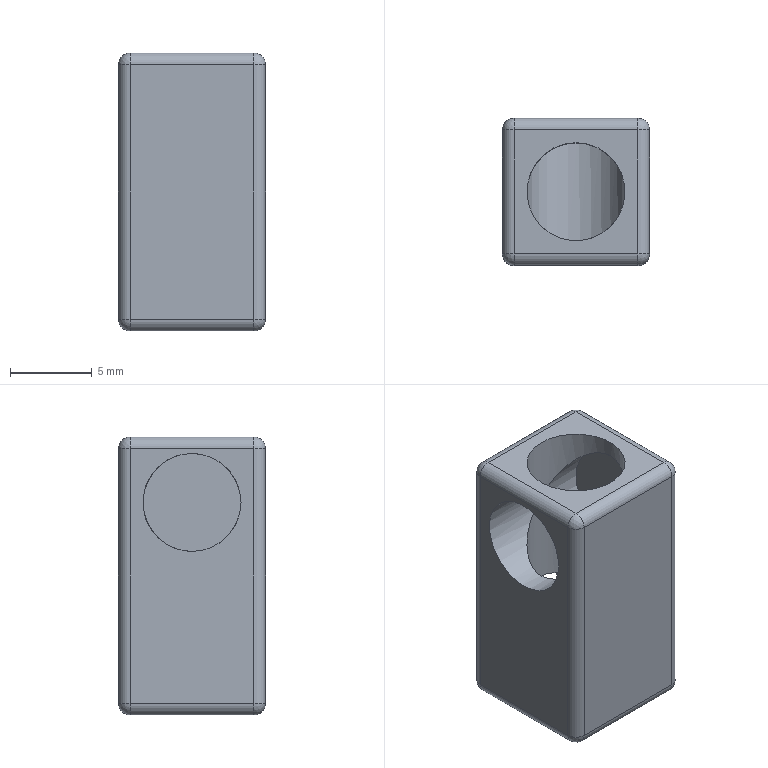Part | STEP file | 1-73.8 | 1 solid | 35 faces | box 9 x 9 x 17 mm | volume 786.768 mm3 | cylinder 19 | plane 8 | sphere 8 | commonest cylinder face diameters 1.414 x12 6 x7